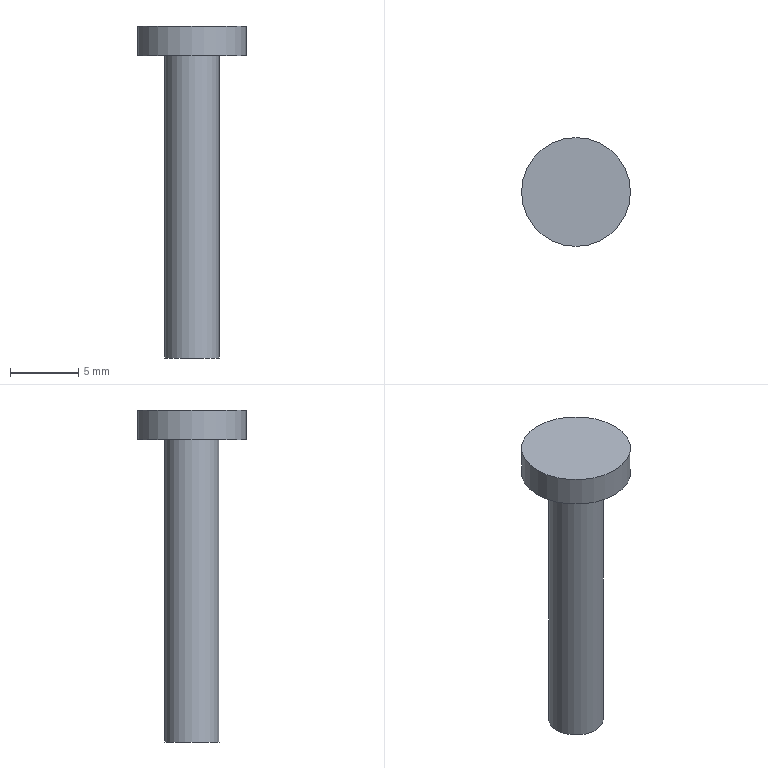Part | NX | features DATUM_CSYS 2, EXTRUDE 2, SKETCH 1 | 1 solid | 5 faces | box 8 x 8 x 24.4 mm | volume 389.557 mm3 | plane 3 | cylinder 2 | commonest cylinder face diameters 4 x1 8 x1
STEP:
#1=CARTESIAN_POINT('',(4.,0.,2.2));
#2=VERTEX_POINT('',#1);
#3=CARTESIAN_POINT('',(0.,0.,2.2));
#4=DIRECTION('',(0.,0.,1.));
#5=DIRECTION('',(1.,0.,0.));
#6=AXIS2_PLACEMENT_3D('',#3,#4,#5);
#7=CIRCLE('',#6,4.);
#8=EDGE_CURVE('',#2,#2,#7,.T.);
#9=ORIENTED_EDGE('',*,*,#8,.F.);
#10=EDGE_LOOP('',(#9));
#11=FACE_BOUND('',#10,.T.);
#12=CARTESIAN_POINT('',(4.,0.,0.));
#13=VERTEX_POINT('',#12);
#14=CARTESIAN_POINT('',(0.,0.,0.));
#15=DIRECTION('',(0.,0.,1.));
#16=DIRECTION('',(1.,0.,0.));
#17=AXIS2_PLACEMENT_3D('',#14,#15,#16);
#18=CIRCLE('',#17,4.);
#19=EDGE_CURVE('',#13,#13,#18,.T.);
#20=ORIENTED_EDGE('',*,*,#19,.T.);
#21=EDGE_LOOP('',(#20));
#22=FACE_BOUND('',#21,.T.);
#23=CARTESIAN_POINT('',(0.,0.,2.2));
#24=DIRECTION('',(0.,0.,-1.));
#25=DIRECTION('',(-1.,0.,0.));
#26=AXIS2_PLACEMENT_3D('',#23,#24,#25);
#27=CYLINDRICAL_SURFACE('',#26,4.);
#28=ADVANCED_FACE('',(#11,#22),#27,.T.);
#29=ORIENTED_EDGE('',*,*,#8,.T.);
#30=EDGE_LOOP('',(#29));
#31=FACE_BOUND('',#30,.T.);
#32=CARTESIAN_POINT('',(0.,0.,2.2));
#33=DIRECTION('',(0.,0.,1.));
#34=DIRECTION('',(1.,0.,0.));
#35=AXIS2_PLACEMENT_3D('',#32,#33,#34);
#36=PLANE('',#35);
#37=ADVANCED_FACE('',(#31),#36,.T.);
#38=CARTESIAN_POINT('',(2.,0.,0.));
#39=VERTEX_POINT('',#38);
#40=CARTESIAN_POINT('',(0.,0.,0.));
#41=DIRECTION('',(0.,0.,-1.));
#42=DIRECTION('',(1.,0.,0.));
#43=AXIS2_PLACEMENT_3D('',#40,#41,#42);
#44=CIRCLE('',#43,2.);
#45=EDGE_CURVE('',#39,#39,#44,.T.);
#46=ORIENTED_EDGE('',*,*,#45,.F.);
#47=EDGE_LOOP('',(#46));
#48=FACE_BOUND('',#47,.T.);
#49=ORIENTED_EDGE('',*,*,#19,.F.);
#50=EDGE_LOOP('',(#49));
#51=FACE_BOUND('',#50,.T.);
#52=CARTESIAN_POINT('',(0.,0.,0.));
#53=DIRECTION('',(0.,0.,1.));
#54=DIRECTION('',(1.,0.,0.));
#55=AXIS2_PLACEMENT_3D('',#52,#53,#54);
#56=PLANE('',#55);
#57=ADVANCED_FACE('',(#48,#51),#56,.F.);
#58=CARTESIAN_POINT('',(2.,0.,-22.2));
#59=VERTEX_POINT('',#58);
#60=CARTESIAN_POINT('',(0.,0.,-22.2));
#61=DIRECTION('',(0.,0.,-1.));
#62=DIRECTION('',(1.,0.,0.));
#63=AXIS2_PLACEMENT_3D('',#60,#61,#62);
#64=CIRCLE('',#63,2.);
#65=EDGE_CURVE('',#59,#59,#64,.T.);
#66=ORIENTED_EDGE('',*,*,#65,.F.);
#67=EDGE_LOOP('',(#66));
#68=FACE_BOUND('',#67,.T.);
#69=ORIENTED_EDGE('',*,*,#45,.T.);
#70=EDGE_LOOP('',(#69));
#71=FACE_BOUND('',#70,.T.);
#72=CARTESIAN_POINT('',(0.,0.,-22.2));
#73=DIRECTION('',(0.,0.,1.));
#74=DIRECTION('',(1.,0.,0.));
#75=AXIS2_PLACEMENT_3D('',#72,#73,#74);
#76=CYLINDRICAL_SURFACE('',#75,2.);
#77=ADVANCED_FACE('',(#68,#71),#76,.T.);
#78=ORIENTED_EDGE('',*,*,#65,.T.);
#79=EDGE_LOOP('',(#78));
#80=FACE_BOUND('',#79,.T.);
#81=CARTESIAN_POINT('',(0.,0.,-22.2));
#82=DIRECTION('',(0.,0.,-1.));
#83=DIRECTION('',(-1.,0.,0.));
#84=AXIS2_PLACEMENT_3D('',#81,#82,#83);
#85=PLANE('',#84);
#86=ADVANCED_FACE('',(#80),#85,.T.);
#87=CLOSED_SHELL('',(#28,#37,#57,#77,#86));
#88=MANIFOLD_SOLID_BREP('',#87);
#89=(LENGTH_UNIT()NAMED_UNIT(*)SI_UNIT(.MILLI.,.METRE.));
#90=UNCERTAINTY_MEASURE_WITH_UNIT(LENGTH_MEASURE(0.00001),#89,'','');
#91=(NAMED_UNIT(*)PLANE_ANGLE_UNIT()SI_UNIT($,.RADIAN.));
#92=(NAMED_UNIT(*)SI_UNIT($,.STERADIAN.)SOLID_ANGLE_UNIT());
#93=(GEOMETRIC_REPRESENTATION_CONTEXT(3)GLOBAL_UNCERTAINTY_ASSIGNED_CONTEXT((#90))GLOBAL_UNIT_ASSIGNED_CONTEXT((#89,#91,#92))REPRESENTATION_CONTEXT('',''));
#94=ADVANCED_BREP_SHAPE_REPRESENTATION('',(#88),#93);